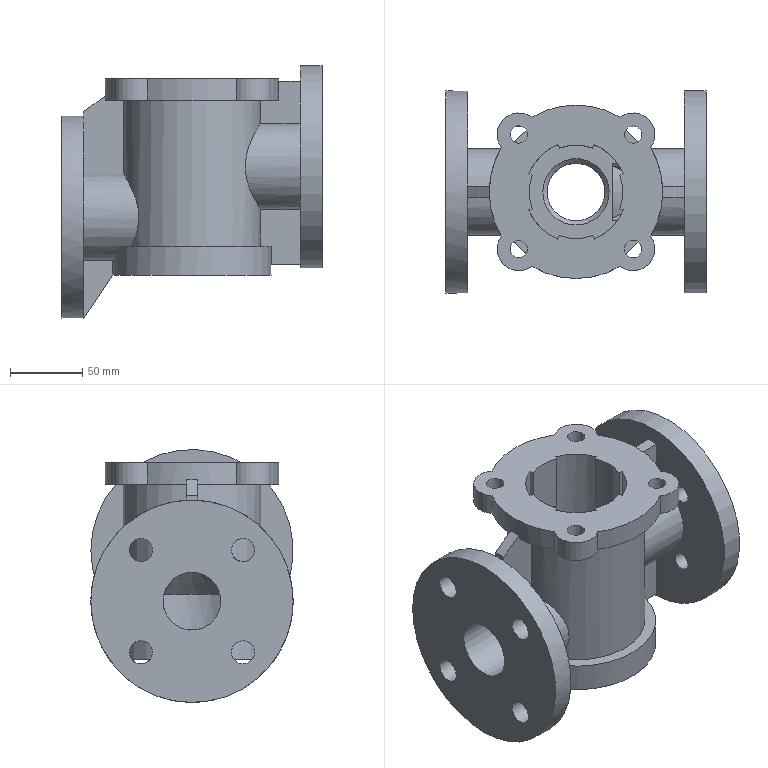Part | NX | features DATUM_CSYS 16, SKETCH 15, EXTRUDE 12, SWP104 7, UNITE 3, PULL_FACE 1 | 1 solid | 89 faces | box 180 x 140 x 175 mm | volume 1165814 mm3 | plane 47 | cylinder 39 | cone 3 | commonest cylinder face diameters 12 x8 16 x4 30 x4 40 x4 60 x4 65 x4